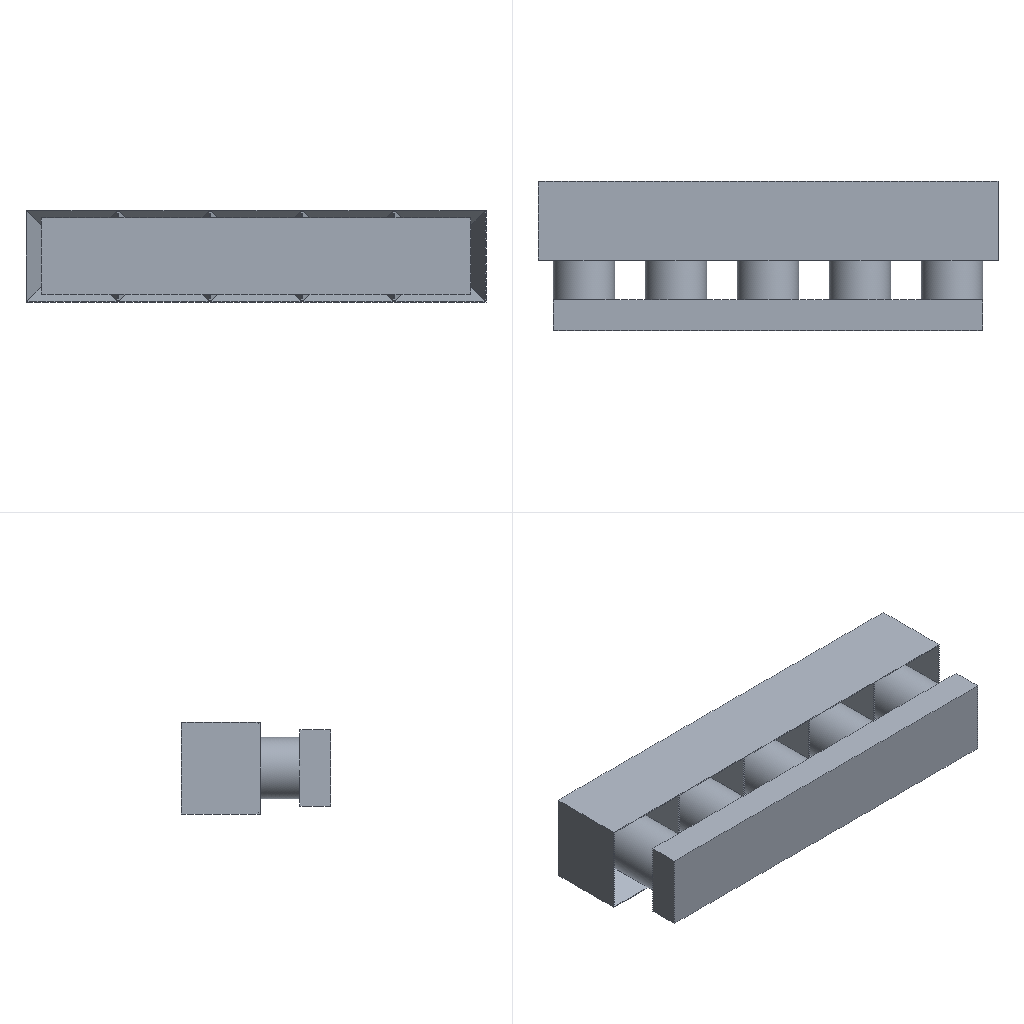Simulation study | ansys workbench
Set-up summary:
category,name,step,type,value,unit,region
solver,ansys_mapdl
solver,version,,,22.1
units,MKS,,stated
analysis,deck,,static,static
load_step,requested,,,1
analysis,nlgeom,,,False
mesh,nodes,,,725865
mesh,elements,,,470595
element_type,ANSYS 187 (type 1),,solid,189480
element_type,ANSYS 187 (type 2),,solid,231613
element_type,ANSYS 174 (type 3),,contact,18202
element_type,ANSYS 170 (type 4),,target,18202
element_type,ANSYS 154 (type 5),,surface,13098
load,load commands in deck,,count,3
bc,support commands in deck,,count,1
named_set,_FIXEDSU,,component
material,1,,in results
material,2,,in results
check,setup vs results,,match,13098 surface effect element(s) are not in the reader's mesh and were not compared
Ansys APDL input file, long lists of numbers shortened:
/batch
/config,noeldb,1     ! force off writing results to database
*get,_wallstrt,active,,time,wall
! ANSYS input file written by Workbench version 2022 R1
! File used for geometry attach: C:\Users\USE\Desktop\微柱@倒金字塔仿真模型\互锁无ppy.x_t
/title,wbnew--____ (A5)
! ****** Begin Custom Load Command Snippet ******
/COM, ACT Extensions:
/COM,     LSDYNA, 2021.1
/COM,
! ****** End   Custom Load Command Snippet ******
*DIM,_wb_ProjectScratch_dir,string,248
_wb_ProjectScratch_dir(1) = 'C:\Users\USE\AppData\Local\Temp\WB_htt_15888_2\_ProjectScratch\ScrB66F\'
*DIM,_wb_SolverFiles_dir,string,248
_wb_SolverFiles_dir(1) = 'C:\Users\USE\AppData\Local\Temp\WB_htt_15888_2\wbnew_files\dp0\SYS\MECH\'
*DIM,_wb_userfiles_dir,string,248
_wb_userfiles_dir(1) = 'C:\Users\USE\AppData\Local\Temp\WB_htt_15888_2\wbnew_files\user_files\'
/com,--- Data in consistent MKS units. See Solving Units in the help system for more information.
/units,MKS
/nopr
/wb,file,start              !  signify a WB generated input file
/prep7
! Turn off shape checking because checks already performed inside WB mesher.
! See help system for more information.
SHPP,OFF,,NOWARN
/nolist
etcon,set             ! allow ANSYS to choose best KEYOP's for 180x elements, resets any applicable keyopt to MAPDL defaults
/com,*********** Nodes for the whole assembly ***********
nblock,3,,798451
(1i9,3e20.9e3)
        1     2.318338027E-01    -4.246774956E-02     6.500000000E-01
! (725864 more lines like these left out)
-1
/wb,elem,start            !  set before creation of elements
/com,*********** Elements for Body 1 "___PPy" ***********
et,1,187
eblock,19,solid,,189480
(19i9)
        1        1        1        1        0        0        0        0       10        0        1    14146    51322    14288    45086   130137   130888   130134   130136
! (378959 more lines like these left out)
-1
/com,*********** Elements for Body 2 "_____PPy" ***********
et,2,187
eblock,19,solid,,231613
(19i9)
        2        2        2        2        0        0        0        0       10        0   189481   362067   389753   380419   389743   586949   697930   586946   586948
! (463225 more lines like these left out)
-1
/wb,elem,end               !  done creating elements
/com,*********** Send User Defined Coordinate System(s) ***********
csys,0
toffst,273.15,  ! Temperature offset from absolute zero
/com,*********** Set Reference Temperature ***********
tref,22.
/wb,mat,start              !  starting to send materials
/com,*********** Send Materials ***********
Temperature = 'TEMP' ! Temperature
MP,DENS,1,1160,	! kg m^-3
MP,EX,1,2303000000,	! Pa
MP,NUXY,1,0.4002,
MP,ALPX,1,9.786e-05,	! C^-1
MP,KXX,1,0.1998,	! W m^-1 C^-1
MP,C,1,1190,	! J kg^-1 C^-1
Temperature = 'TEMP' ! Temperature
MP,DENS,2,1160,	! kg m^-3
MP,EX,2,2303000000,	! Pa
MP,NUXY,2,0.4002,
MP,ALPX,2,9.786e-05,	! C^-1
MP,KXX,2,0.1998,	! W m^-1 C^-1
MP,C,2,1190,	! J kg^-1 C^-1
/wb,mat,end                !  done sending materials
!************************* Model Summary ********************
!___PPy,	塑性，PC（共聚物，耐热）,	matid,	1
!_____PPy,	塑性，PC（共聚物，耐热）,	matid,	2
!************************* End Model Summary ********************
! get the diagonal of the bounding box. Needed later for other things
*get,_xmin,node,,mnloc,x
*get,_ymin,node,,mnloc,y
*get,_zmin,node,,mnloc,z
*get,_xmax,node,,mxloc,x
*get,_ymax,node,,mxloc,y
*get,_zmax,node,,mxloc,z
_ASMDIAG=(_xmax-_xmin)*(_xmax-_xmin)+(_ymax-_ymin)*(_ymax-_ymin)+(_zmax-_zmin)*(_zmax-_zmin)
_ASMDIAG=SQRT(_ASMDIAG)
/wb,contact,start          !  starting to send contact
/com,*********** Create Contact "接触区域" ***********
/com,            Real Constant Set For Above Contact Is 4 & 3
*set,tid,4
*set,cid,3
r,tid
r,cid
et,tid,170
et,cid,174
eblock,10,,,9463
(15i9)
   578906        4        4        4        0     1749     1750     7720     7720    63695    63703     7720    63696
! (9462 more lines like these left out)
-1
eblock,10,,,9463
(15i9)
   588369        3        3        3        0     1749     1750     7720     7720    63695    63703     7720    63696
! (9462 more lines like these left out)
-1
eblock,10,,,8739
(15i9)
   597832        3        4        3        0   370229   370905   370725   370725   627451   630734   370725   627448
! (8738 more lines like these left out)
-1
eblock,10,,,8739
(15i9)
   606571        4        3        4        0   370229   370905   370725   370725   627451   630734   370725   627448
! (8738 more lines like these left out)
-1
keyo,cid,8,2               ! auto create asymmetric contact (from Program Controlled setting)
keyo,cid,10,0              ! adjust contact stiffness each NR iteration (from Program Controlled setting)
keyo,cid,12,5              ! bonded always
keyo,cid,18,1              ! small sliding turned on by application
keyo,cid,2,0               ! augmented Lagrange (from Program Controlled setting)
keyo,cid,4,0               ! on Gauss point (from Program Controlled setting)
keyo,cid,9,1               ! ignore initial gaps/penetration
keyo,cid,7,0               ! No Prediction
rmod,tid,3,10.      ! FKN
rmod,tid,5,0.       ! ICONT
rmod,tid,6,0.       ! PINB
rmod,tid,10,0.      ! CNOF
rmod,tid,12,0.      ! FKT
rmod,tid,36,30      ! WB DSID
rmod,cid,3,10.      ! FKN
rmod,cid,5,0.       ! ICONT
rmod,cid,6,0.       ! PINB
rmod,cid,10,0.      ! CNOF
rmod,cid,12,0.      ! FKT
rmod,cid,36,30      ! WB DSID
nsel,all
esel,all
/wb,contact,end            !  done creating contacts
/golist
/wb,load,start             !  starting to send loads
/com,*********** Fixed Supports ***********
CMBLOCK,_FIXEDSU,NODE,   100069
(8i10)
    329094    329095    329096    329097    329098    329099    329100    329101
! (12508 more lines like these left out)
cmsel,s,_FIXEDSU
d,all,all
nsel,all
/com,*********** Define Force Using Surface Effect Elements ***********
local,12,0,0.,0.,0.,0.,0.,0.
csys,0
et,5,154
eblock,10,,,13098
(15i9)
   615310        5        5        5       12    25541    26101    27643    27643   192925   197792    27643   192927
! (13097 more lines like these left out)
-1
esel,s,type,,5
keyop,5,2,1                ! Apply load in local coordinate system
keyop,5,7,1                ! Use original area so load is constant in large deformation
esel,all
/gst,on,on
fini
*get,_numnode,node,0,count
*get,_numelem,elem,0,count
*get, _MAXELEMNUM, elem, 0, NUM, MAX
*get, _MAXNODENUM, node, 0, NUM, MAX
*get, _MAXELEMTYPE, etyp, 0, NUM, MAX
*get, _MAXREALCONST, real, 0, NUM, MAX
/go
/wb,load,end               !  done creating loads
/com,--- Number of total nodes = %_numnode%
/com,--- Number of contact elements = 49502
/com,--- Number of spring elements = 0
/com,--- Number of bearing elements = 0
/com,--- Number of solid elements = 421093
/com,--- Number of condensed parts = 0
/com,--- Number of total elements = %_numelem%
*get,_wallbsol,active,,time,wall
/com,****************************************************************************
/com,*************************    SOLUTION       ********************************
/com,****************************************************************************
/solu
antype,0                   ! static analysis
_thickRatio=  1     ! Ratio of thick parts in the model
eqsl,pcg,1e-8,,,,,,1
cntr,print,1               ! print out contact info and also make no initial contact an error
dmpoption,emat,no             ! Don't combine emat file for DANSYS
dmpoption,esav,no             ! Don't combine esav file for DANSYS
nldiag,cont,iter           ! print out contact info each equilibrium iteration
rescontrol,,none                 ! Do not keep any restart files
/com,****************************************************
/com,******************* SOLVE FOR LS 1 OF 1 ****************
esel,s,type,,5
nsle
sfe,all,1,pres,1,0.
sfe,all,2,pres,1,178.571
sfe,all,3,pres,1,0.
nsel,all
esel,all
/nopr
/gopr
nsub,1,1,1
time,1.
outres,erase
outres,all,none
outres,nsol,all,
outres,rsol,all
outres,eangl,all
outres,etmp,all
outres,veng,all
outres,strs,all,
outres,epel,all,
outres,eppl,all,
outres,cont,all,
! *********** WB SOLVE COMMAND ***********
! check interactive state
*get,ANSINTER_,active,,int
*if,ANSINTER_,ne,0,then
/eof
*endif
solve
/com *************** Write FE CONNECTORS *********
CEWRITE,file,ce,,INTE
/com,****************************************************
/com,*************** FINISHED SOLVE FOR LS 1 *************
*get,_wallasol,active,,time,wall
/nopr
*get,_numnode,node,0,count
*get,_numelem,elem,0,count
*get, _MAXELEMNUM, elem, 0, NUM, MAX
*get, _MAXNODENUM, node, 0, NUM, MAX,,,INTERNAL
*get, _MAXELEMTYPE, etyp, 0, NUM, MAX
*get, _MAXREALCONST, real, 0, NUM, MAX
/gopr
*get,_PCGITER,active,,solu,cgiter
/post1
xmlo,ENCODING,ISO-8859-1
xmlo,parm
/xml,parm,xml
fini
/gopr
*get,_walldone,active,,time,wall
_preptime=(_wallbsol-_wallstrt)*3600
_solvtime=(_wallasol-_wallbsol)*3600
_posttime=(_walldone-_wallasol)*3600
_totaltim=(_walldone-_wallstrt)*3600
*get,_dlbratio,active,0,solu,dlbr
*get,_combtime,active,0,solu,comb
*get,_ssmode,active,0,solu,ssmm
*get,_ndofs,active,0,solu,ndof
*get,_sol_end_time,active,0,set,time
*if,_sol_end_time,eq,1.,then
/fclean				!clean distributed files
*endif
/com,--- Total number of nodes = %_numnode%
/com,--- Total number of elements = %_numelem%
/com,--- Element load balance ratio = %_dlbratio%
/com,--- Time to combine distributed files = %_combtime%
/com,--- Sparse memory mode = %_ssmode%
/com,--- Number of DOF = %_ndofs%
/wb,file,end               ! done with WB generated input
Results summary:
result,analysis,,,static
result,last_loadstep,,,1
result,primary field,,,displacement
result,reaction total,1,FX,-0.0,N
result,reaction total,1,FY,-10.0,N
result,reaction total,1,FZ,-0.0,N
result,mass,,,11.15,"MKS: m, kg, N, s, V, A, degC"